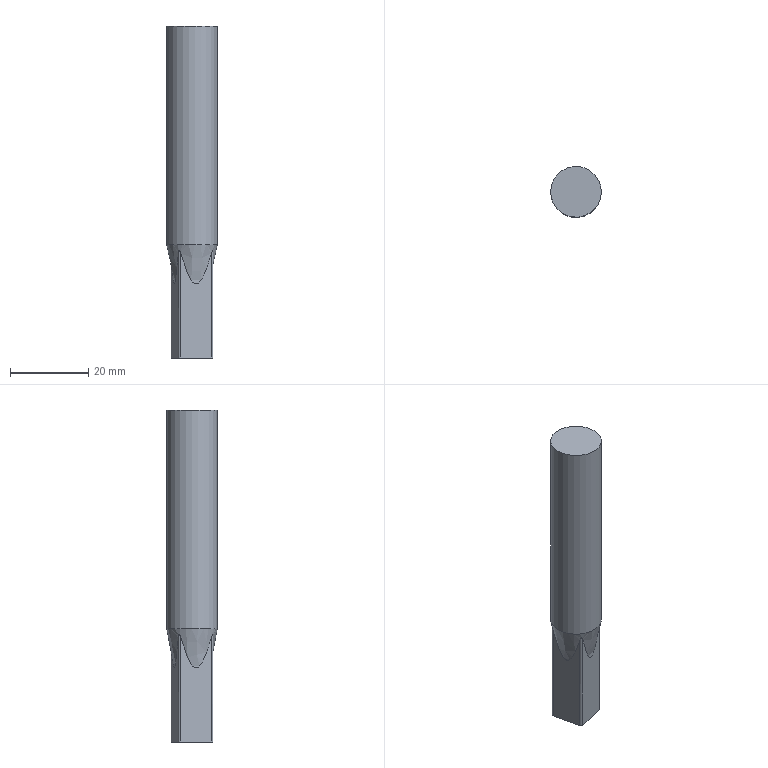Part | NX | features solid 2 | 1 solid | 12 faces | box 13 x 13 x 85 mm | volume 10020 mm3 | plane 6 | cylinder 5 | cone 1 | commonest cylinder face diameters 1.1 x4 13 x1
STEP:
#1=CARTESIAN_POINT('',(-690.242,-351.357,51.));
#2=VERTEX_POINT('',#1);
#3=CARTESIAN_POINT('',(-682.453,-349.534,51.));
#4=VERTEX_POINT('',#3);
#5=CARTESIAN_POINT('',(-686.347,-350.445,51.));
#6=DIRECTION('',(0.9737,0.2278,0.));
#7=VECTOR('',#6,1000.);
#8=LINE('',#5,#7);
#9=EDGE_CURVE('',#2,#4,#8,.T.);
#10=ORIENTED_EDGE('',*,*,#9,.T.);
#11=CARTESIAN_POINT('',(-682.453,-349.534,77.735));
#12=VERTEX_POINT('',#11);
#13=CARTESIAN_POINT('',(-682.453,-349.534,51.));
#14=DIRECTION('',(0.,0.,1.));
#15=VECTOR('',#14,1000.);
#16=LINE('',#13,#15);
#17=EDGE_CURVE('',#4,#12,#16,.T.);
#18=ORIENTED_EDGE('',*,*,#17,.T.);
#19=CARTESIAN_POINT('',(-690.242,-351.357,77.735));
#20=VERTEX_POINT('',#19);
#21=CARTESIAN_POINT('',(-690.242,-351.357,77.735));
#22=CARTESIAN_POINT('',(-690.035,-351.308,77.013));
#23=CARTESIAN_POINT('',(-689.603,-351.207,75.574));
#24=CARTESIAN_POINT('',(-688.992,-351.064,73.795));
#25=CARTESIAN_POINT('',(-688.427,-350.932,72.408));
#26=CARTESIAN_POINT('',(-687.922,-350.814,71.396));
#27=CARTESIAN_POINT('',(-687.342,-350.678,70.456));
#28=CARTESIAN_POINT('',(-686.302,-350.435,69.756));
#29=CARTESIAN_POINT('',(-685.305,-350.201,70.527));
#30=CARTESIAN_POINT('',(-684.739,-350.069,71.456));
#31=CARTESIAN_POINT('',(-684.242,-349.953,72.469));
#32=CARTESIAN_POINT('',(-683.686,-349.823,73.841));
#33=CARTESIAN_POINT('',(-683.085,-349.682,75.597));
#34=CARTESIAN_POINT('',(-682.658,-349.582,77.02));
#35=CARTESIAN_POINT('',(-682.453,-349.534,77.735));
#36=B_SPLINE_CURVE_WITH_KNOTS('',3,(#21,#22,#23,#24,#25,#26,#27,#28,#29,#30,#31,#32,#33,#34,#35),.UNSPECIFIED.,.F.,.F.,(4,1,1,1,1,1,1,1,1,1,1,1,4),(0.002007,0.004266,0.006525,0.007654,0.008784,0.009913,0.01104,0.01217,0.0133,0.01443,0.01556,0.01782,0.02008),.UNSPECIFIED.);
#37=EDGE_CURVE('',#20,#12,#36,.T.);
#38=ORIENTED_EDGE('',*,*,#37,.F.);
#39=CARTESIAN_POINT('',(-690.242,-351.357,51.));
#40=DIRECTION('',(0.,0.,1.));
#41=VECTOR('',#40,1000.);
#42=LINE('',#39,#41);
#43=EDGE_CURVE('',#20,#2,#42,.F.);
#44=ORIENTED_EDGE('',*,*,#43,.T.);
#45=EDGE_LOOP('',(#10,#18,#38,#44));
#46=FACE_BOUND('',#45,.T.);
#47=CARTESIAN_POINT('',(-686.347,-350.445,51.));
#48=DIRECTION('',(0.2278,-0.9737,0.));
#49=DIRECTION('',(0.,0.,-1.));
#50=AXIS2_PLACEMENT_3D('',#47,#48,#49);
#51=PLANE('',#50);
#52=ADVANCED_FACE('',(#46),#51,.T.);
#53=CARTESIAN_POINT('',(-692.726,-343.157,77.735));
#54=VERTEX_POINT('',#53);
#55=CARTESIAN_POINT('',(-690.903,-350.946,77.735));
#56=VERTEX_POINT('',#55);
#57=CARTESIAN_POINT('',(-692.726,-343.157,77.735));
#58=CARTESIAN_POINT('',(-692.677,-343.364,77.013));
#59=CARTESIAN_POINT('',(-692.576,-343.796,75.574));
#60=CARTESIAN_POINT('',(-692.433,-344.407,73.795));
#61=CARTESIAN_POINT('',(-692.301,-344.972,72.408));
#62=CARTESIAN_POINT('',(-692.183,-345.477,71.396));
#63=CARTESIAN_POINT('',(-692.047,-346.057,70.456));
#64=CARTESIAN_POINT('',(-691.804,-347.096,69.756));
#65=CARTESIAN_POINT('',(-691.57,-348.094,70.527));
#66=CARTESIAN_POINT('',(-691.438,-348.66,71.456));
#67=CARTESIAN_POINT('',(-691.322,-349.157,72.469));
#68=CARTESIAN_POINT('',(-691.192,-349.713,73.841));
#69=CARTESIAN_POINT('',(-691.051,-350.314,75.597));
#70=CARTESIAN_POINT('',(-690.951,-350.741,77.02));
#71=CARTESIAN_POINT('',(-690.903,-350.946,77.735));
#72=B_SPLINE_CURVE_WITH_KNOTS('',3,(#57,#58,#59,#60,#61,#62,#63,#64,#65,#66,#67,#68,#69,#70,#71),.UNSPECIFIED.,.F.,.F.,(4,1,1,1,1,1,1,1,1,1,1,1,4),(0.002007,0.004266,0.006525,0.007654,0.008784,0.009913,0.01104,0.01217,0.0133,0.01443,0.01556,0.01782,0.02008),.UNSPECIFIED.);
#73=EDGE_CURVE('',#54,#56,#72,.T.);
#74=ORIENTED_EDGE('',*,*,#73,.F.);
#75=CARTESIAN_POINT('',(-692.726,-343.157,51.));
#76=VERTEX_POINT('',#75);
#77=CARTESIAN_POINT('',(-692.726,-343.157,51.));
#78=DIRECTION('',(0.,0.,1.));
#79=VECTOR('',#78,1000.);
#80=LINE('',#77,#79);
#81=EDGE_CURVE('',#54,#76,#80,.F.);
#82=ORIENTED_EDGE('',*,*,#81,.T.);
#83=CARTESIAN_POINT('',(-690.903,-350.946,51.));
#84=VERTEX_POINT('',#83);
#85=CARTESIAN_POINT('',(-691.814,-347.052,51.));
#86=DIRECTION('',(0.2278,-0.9737,0.));
#87=VECTOR('',#86,1000.);
#88=LINE('',#85,#87);
#89=EDGE_CURVE('',#76,#84,#88,.T.);
#90=ORIENTED_EDGE('',*,*,#89,.T.);
#91=CARTESIAN_POINT('',(-690.903,-350.946,51.));
#92=DIRECTION('',(0.,0.,1.));
#93=VECTOR('',#92,1000.);
#94=LINE('',#91,#93);
#95=EDGE_CURVE('',#84,#56,#94,.T.);
#96=ORIENTED_EDGE('',*,*,#95,.T.);
#97=EDGE_LOOP('',(#74,#82,#90,#96));
#98=FACE_BOUND('',#97,.T.);
#99=CARTESIAN_POINT('',(-691.814,-347.052,51.));
#100=DIRECTION('',(-0.9737,-0.2278,0.));
#101=DIRECTION('',(0.,0.,1.));
#102=AXIS2_PLACEMENT_3D('',#99,#100,#101);
#103=PLANE('',#102);
#104=ADVANCED_FACE('',(#98),#103,.T.);
#105=CARTESIAN_POINT('',(-684.526,-340.673,77.735));
#106=VERTEX_POINT('',#105);
#107=CARTESIAN_POINT('',(-692.315,-342.496,77.735));
#108=VERTEX_POINT('',#107);
#109=CARTESIAN_POINT('',(-684.526,-340.673,77.735));
#110=CARTESIAN_POINT('',(-684.733,-340.722,77.013));
#111=CARTESIAN_POINT('',(-685.165,-340.823,75.574));
#112=CARTESIAN_POINT('',(-685.776,-340.966,73.795));
#113=CARTESIAN_POINT('',(-686.341,-341.098,72.408));
#114=CARTESIAN_POINT('',(-686.846,-341.216,71.396));
#115=CARTESIAN_POINT('',(-687.426,-341.352,70.456));
#116=CARTESIAN_POINT('',(-688.465,-341.595,69.756));
#117=CARTESIAN_POINT('',(-689.463,-341.829,70.527));
#118=CARTESIAN_POINT('',(-690.029,-341.961,71.456));
#119=CARTESIAN_POINT('',(-690.526,-342.077,72.469));
#120=CARTESIAN_POINT('',(-691.082,-342.207,73.841));
#121=CARTESIAN_POINT('',(-691.683,-342.348,75.597));
#122=CARTESIAN_POINT('',(-692.11,-342.448,77.02));
#123=CARTESIAN_POINT('',(-692.315,-342.496,77.735));
#124=B_SPLINE_CURVE_WITH_KNOTS('',3,(#109,#110,#111,#112,#113,#114,#115,#116,#117,#118,#119,#120,#121,#122,#123),.UNSPECIFIED.,.F.,.F.,(4,1,1,1,1,1,1,1,1,1,1,1,4),(0.002007,0.004266,0.006525,0.007654,0.008784,0.009913,0.01104,0.01217,0.0133,0.01443,0.01556,0.01782,0.02008),.UNSPECIFIED.);
#125=EDGE_CURVE('',#106,#108,#124,.T.);
#126=ORIENTED_EDGE('',*,*,#125,.F.);
#127=CARTESIAN_POINT('',(-684.526,-340.673,51.));
#128=VERTEX_POINT('',#127);
#129=CARTESIAN_POINT('',(-684.526,-340.673,51.));
#130=DIRECTION('',(0.,0.,1.));
#131=VECTOR('',#130,1000.);
#132=LINE('',#129,#131);
#133=EDGE_CURVE('',#106,#128,#132,.F.);
#134=ORIENTED_EDGE('',*,*,#133,.T.);
#135=CARTESIAN_POINT('',(-692.315,-342.496,51.));
#136=VERTEX_POINT('',#135);
#137=CARTESIAN_POINT('',(-688.421,-341.585,51.));
#138=DIRECTION('',(-0.9737,-0.2278,0.));
#139=VECTOR('',#138,1000.);
#140=LINE('',#137,#139);
#141=EDGE_CURVE('',#128,#136,#140,.T.);
#142=ORIENTED_EDGE('',*,*,#141,.T.);
#143=CARTESIAN_POINT('',(-692.315,-342.496,51.));
#144=DIRECTION('',(0.,0.,1.));
#145=VECTOR('',#144,1000.);
#146=LINE('',#143,#145);
#147=EDGE_CURVE('',#136,#108,#146,.T.);
#148=ORIENTED_EDGE('',*,*,#147,.T.);
#149=EDGE_LOOP('',(#126,#134,#142,#148));
#150=FACE_BOUND('',#149,.T.);
#151=CARTESIAN_POINT('',(-688.421,-341.585,51.));
#152=DIRECTION('',(-0.2278,0.9737,0.));
#153=DIRECTION('',(0.,0.,1.));
#154=AXIS2_PLACEMENT_3D('',#151,#152,#153);
#155=PLANE('',#154);
#156=ADVANCED_FACE('',(#150),#155,.T.);
#157=CARTESIAN_POINT('',(-682.042,-348.873,51.));
#158=VERTEX_POINT('',#157);
#159=CARTESIAN_POINT('',(-683.865,-341.084,51.));
#160=VERTEX_POINT('',#159);
#161=CARTESIAN_POINT('',(-682.954,-344.978,51.));
#162=DIRECTION('',(-0.2278,0.9737,0.));
#163=VECTOR('',#162,1000.);
#164=LINE('',#161,#163);
#165=EDGE_CURVE('',#158,#160,#164,.T.);
#166=ORIENTED_EDGE('',*,*,#165,.F.);
#167=CARTESIAN_POINT('',(-682.578,-348.998,51.));
#168=DIRECTION('',(0.,0.,-1.));
#169=DIRECTION('',(-1.,0.,0.));
#170=AXIS2_PLACEMENT_3D('',#167,#168,#169);
#171=CIRCLE('',#170,0.55);
#172=EDGE_CURVE('',#158,#4,#171,.T.);
#173=ORIENTED_EDGE('',*,*,#172,.T.);
#174=ORIENTED_EDGE('',*,*,#9,.F.);
#175=CARTESIAN_POINT('',(-690.367,-350.821,51.));
#176=DIRECTION('',(0.,0.,-1.));
#177=DIRECTION('',(-1.,0.,0.));
#178=AXIS2_PLACEMENT_3D('',#175,#176,#177);
#179=CIRCLE('',#178,0.55);
#180=EDGE_CURVE('',#2,#84,#179,.T.);
#181=ORIENTED_EDGE('',*,*,#180,.T.);
#182=ORIENTED_EDGE('',*,*,#89,.F.);
#183=CARTESIAN_POINT('',(-692.19,-343.031,51.));
#184=DIRECTION('',(0.,0.,-1.));
#185=DIRECTION('',(-1.,0.,0.));
#186=AXIS2_PLACEMENT_3D('',#183,#184,#185);
#187=CIRCLE('',#186,0.55);
#188=EDGE_CURVE('',#76,#136,#187,.T.);
#189=ORIENTED_EDGE('',*,*,#188,.T.);
#190=ORIENTED_EDGE('',*,*,#141,.F.);
#191=CARTESIAN_POINT('',(-684.4,-341.209,51.));
#192=DIRECTION('',(0.,0.,-1.));
#193=DIRECTION('',(-1.,0.,0.));
#194=AXIS2_PLACEMENT_3D('',#191,#192,#193);
#195=CIRCLE('',#194,0.55);
#196=EDGE_CURVE('',#128,#160,#195,.T.);
#197=ORIENTED_EDGE('',*,*,#196,.T.);
#198=EDGE_LOOP('',(#166,#173,#174,#181,#182,#189,#190,#197));
#199=FACE_BOUND('',#198,.T.);
#200=CARTESIAN_POINT('',(-687.384,-346.015,51.));
#201=DIRECTION('',(0.,0.,-1.));
#202=DIRECTION('',(-0.9737,-0.2278,0.));
#203=AXIS2_PLACEMENT_3D('',#200,#201,#202);
#204=PLANE('',#203);
#205=ADVANCED_FACE('',(#199),#204,.T.);
#206=CARTESIAN_POINT('',(-682.042,-348.873,77.735));
#207=VERTEX_POINT('',#206);
#208=CARTESIAN_POINT('',(-683.865,-341.084,77.735));
#209=VERTEX_POINT('',#208);
#210=CARTESIAN_POINT('',(-682.042,-348.873,77.735));
#211=CARTESIAN_POINT('',(-682.091,-348.666,77.013));
#212=CARTESIAN_POINT('',(-682.192,-348.234,75.574));
#213=CARTESIAN_POINT('',(-682.335,-347.623,73.795));
#214=CARTESIAN_POINT('',(-682.467,-347.058,72.408));
#215=CARTESIAN_POINT('',(-682.585,-346.553,71.396));
#216=CARTESIAN_POINT('',(-682.721,-345.973,70.456));
#217=CARTESIAN_POINT('',(-682.964,-344.933,69.756));
#218=CARTESIAN_POINT('',(-683.198,-343.936,70.527));
#219=CARTESIAN_POINT('',(-683.33,-343.37,71.456));
#220=CARTESIAN_POINT('',(-683.446,-342.873,72.469));
#221=CARTESIAN_POINT('',(-683.576,-342.317,73.841));
#222=CARTESIAN_POINT('',(-683.717,-341.716,75.597));
#223=CARTESIAN_POINT('',(-683.817,-341.289,77.02));
#224=CARTESIAN_POINT('',(-683.865,-341.084,77.735));
#225=B_SPLINE_CURVE_WITH_KNOTS('',3,(#210,#211,#212,#213,#214,#215,#216,#217,#218,#219,#220,#221,#222,#223,#224),.UNSPECIFIED.,.F.,.F.,(4,1,1,1,1,1,1,1,1,1,1,1,4),(0.002007,0.004266,0.006525,0.007654,0.008784,0.009913,0.01104,0.01217,0.0133,0.01443,0.01556,0.01782,0.02008),.UNSPECIFIED.);
#226=EDGE_CURVE('',#207,#209,#225,.T.);
#227=ORIENTED_EDGE('',*,*,#226,.F.);
#228=CARTESIAN_POINT('',(-682.042,-348.873,51.));
#229=DIRECTION('',(0.,0.,1.));
#230=VECTOR('',#229,1000.);
#231=LINE('',#228,#230);
#232=EDGE_CURVE('',#207,#158,#231,.F.);
#233=ORIENTED_EDGE('',*,*,#232,.T.);
#234=ORIENTED_EDGE('',*,*,#165,.T.);
#235=CARTESIAN_POINT('',(-683.865,-341.084,51.));
#236=DIRECTION('',(0.,0.,1.));
#237=VECTOR('',#236,1000.);
#238=LINE('',#235,#237);
#239=EDGE_CURVE('',#160,#209,#238,.T.);
#240=ORIENTED_EDGE('',*,*,#239,.T.);
#241=EDGE_LOOP('',(#227,#233,#234,#240));
#242=FACE_BOUND('',#241,.T.);
#243=CARTESIAN_POINT('',(-682.954,-344.978,51.));
#244=DIRECTION('',(0.9737,0.2278,0.));
#245=DIRECTION('',(0.,0.,-1.));
#246=AXIS2_PLACEMENT_3D('',#243,#244,#245);
#247=PLANE('',#246);
#248=ADVANCED_FACE('',(#242),#247,.T.);
#249=ORIENTED_EDGE('',*,*,#226,.T.);
#250=CARTESIAN_POINT('',(-683.865,-341.084,77.735));
#251=CARTESIAN_POINT('',(-683.875,-341.042,77.881));
#252=CARTESIAN_POINT('',(-683.901,-340.971,78.1));
#253=CARTESIAN_POINT('',(-683.962,-340.866,78.368));
#254=CARTESIAN_POINT('',(-684.105,-340.728,78.562));
#255=CARTESIAN_POINT('',(-684.29,-340.664,78.363));
#256=CARTESIAN_POINT('',(-684.409,-340.656,78.099));
#257=CARTESIAN_POINT('',(-684.484,-340.664,77.88));
#258=CARTESIAN_POINT('',(-684.526,-340.673,77.735));
#259=B_SPLINE_CURVE_WITH_KNOTS('',3,(#250,#251,#252,#253,#254,#255,#256,#257,#258),.UNSPECIFIED.,.F.,.F.,(4,1,1,1,1,1,4),(0.,0.0004558,0.0006837,0.0009116,0.001139,0.001367,0.001823),.UNSPECIFIED.);
#260=EDGE_CURVE('',#209,#106,#259,.T.);
#261=ORIENTED_EDGE('',*,*,#260,.T.);
#262=ORIENTED_EDGE('',*,*,#125,.T.);
#263=CARTESIAN_POINT('',(-692.315,-342.496,77.735));
#264=CARTESIAN_POINT('',(-692.357,-342.506,77.881));
#265=CARTESIAN_POINT('',(-692.428,-342.532,78.1));
#266=CARTESIAN_POINT('',(-692.533,-342.593,78.368));
#267=CARTESIAN_POINT('',(-692.671,-342.736,78.562));
#268=CARTESIAN_POINT('',(-692.735,-342.921,78.363));
#269=CARTESIAN_POINT('',(-692.743,-343.04,78.099));
#270=CARTESIAN_POINT('',(-692.735,-343.115,77.88));
#271=CARTESIAN_POINT('',(-692.726,-343.157,77.735));
#272=B_SPLINE_CURVE_WITH_KNOTS('',3,(#263,#264,#265,#266,#267,#268,#269,#270,#271),.UNSPECIFIED.,.F.,.F.,(4,1,1,1,1,1,4),(0.,0.0004558,0.0006837,0.0009116,0.001139,0.001367,0.001823),.UNSPECIFIED.);
#273=EDGE_CURVE('',#108,#54,#272,.T.);
#274=ORIENTED_EDGE('',*,*,#273,.T.);
#275=ORIENTED_EDGE('',*,*,#73,.T.);
#276=CARTESIAN_POINT('',(-690.903,-350.946,77.735));
#277=CARTESIAN_POINT('',(-690.893,-350.988,77.881));
#278=CARTESIAN_POINT('',(-690.867,-351.059,78.1));
#279=CARTESIAN_POINT('',(-690.806,-351.164,78.368));
#280=CARTESIAN_POINT('',(-690.663,-351.302,78.562));
#281=CARTESIAN_POINT('',(-690.478,-351.366,78.363));
#282=CARTESIAN_POINT('',(-690.359,-351.374,78.099));
#283=CARTESIAN_POINT('',(-690.284,-351.366,77.88));
#284=CARTESIAN_POINT('',(-690.242,-351.357,77.735));
#285=B_SPLINE_CURVE_WITH_KNOTS('',3,(#276,#277,#278,#279,#280,#281,#282,#283,#284),.UNSPECIFIED.,.F.,.F.,(4,1,1,1,1,1,4),(0.,0.0004558,0.0006837,0.0009116,0.001139,0.001367,0.001823),.UNSPECIFIED.);
#286=EDGE_CURVE('',#56,#20,#285,.T.);
#287=ORIENTED_EDGE('',*,*,#286,.T.);
#288=ORIENTED_EDGE('',*,*,#37,.T.);
#289=CARTESIAN_POINT('',(-682.453,-349.534,77.735));
#290=CARTESIAN_POINT('',(-682.411,-349.524,77.881));
#291=CARTESIAN_POINT('',(-682.34,-349.498,78.1));
#292=CARTESIAN_POINT('',(-682.235,-349.437,78.368));
#293=CARTESIAN_POINT('',(-682.097,-349.294,78.562));
#294=CARTESIAN_POINT('',(-682.033,-349.109,78.363));
#295=CARTESIAN_POINT('',(-682.025,-348.99,78.099));
#296=CARTESIAN_POINT('',(-682.033,-348.915,77.88));
#297=CARTESIAN_POINT('',(-682.042,-348.873,77.735));
#298=B_SPLINE_CURVE_WITH_KNOTS('',3,(#289,#290,#291,#292,#293,#294,#295,#296,#297),.UNSPECIFIED.,.F.,.F.,(4,1,1,1,1,1,4),(0.,0.0004558,0.0006837,0.0009116,0.001139,0.001367,0.001823),.UNSPECIFIED.);
#299=EDGE_CURVE('',#12,#207,#298,.T.);
#300=ORIENTED_EDGE('',*,*,#299,.T.);
#301=EDGE_LOOP('',(#249,#261,#262,#274,#275,#287,#288,#300));
#302=FACE_BOUND('',#301,.T.);
#303=CARTESIAN_POINT('',(-681.055,-344.534,80.));
#304=VERTEX_POINT('',#303);
#305=CARTESIAN_POINT('',(-687.384,-346.015,80.));
#306=DIRECTION('',(0.,0.,1.));
#307=DIRECTION('',(0.9737,0.2278,0.));
#308=AXIS2_PLACEMENT_3D('',#305,#306,#307);
#309=CIRCLE('',#308,6.5);
#310=EDGE_CURVE('',#304,#304,#309,.T.);
#311=ORIENTED_EDGE('',*,*,#310,.F.);
#312=EDGE_LOOP('',(#311));
#313=FACE_BOUND('',#312,.T.);
#314=CARTESIAN_POINT('',(-687.384,-346.015,70.));
#315=DIRECTION('',(0.,0.,1.));
#316=DIRECTION('',(0.9737,0.2278,0.));
#317=AXIS2_PLACEMENT_3D('',#314,#315,#316);
#318=CONICAL_SURFACE('',#317,4.55,0.1926);
#319=ADVANCED_FACE('',(#302,#313),#318,.T.);
#320=CARTESIAN_POINT('',(-693.713,-347.496,136.));
#321=VERTEX_POINT('',#320);
#322=CARTESIAN_POINT('',(-687.384,-346.015,136.));
#323=DIRECTION('',(0.,0.,-1.));
#324=DIRECTION('',(-0.9737,-0.2278,0.));
#325=AXIS2_PLACEMENT_3D('',#322,#323,#324);
#326=CIRCLE('',#325,6.5);
#327=EDGE_CURVE('',#321,#321,#326,.T.);
#328=ORIENTED_EDGE('',*,*,#327,.F.);
#329=EDGE_LOOP('',(#328));
#330=FACE_BOUND('',#329,.T.);
#331=CARTESIAN_POINT('',(-687.384,-346.015,136.));
#332=DIRECTION('',(0.,0.,1.));
#333=DIRECTION('',(0.9737,0.2278,0.));
#334=AXIS2_PLACEMENT_3D('',#331,#332,#333);
#335=PLANE('',#334);
#336=ADVANCED_FACE('',(#330),#335,.T.);
#337=ORIENTED_EDGE('',*,*,#327,.T.);
#338=EDGE_LOOP('',(#337));
#339=FACE_BOUND('',#338,.T.);
#340=ORIENTED_EDGE('',*,*,#310,.T.);
#341=EDGE_LOOP('',(#340));
#342=FACE_BOUND('',#341,.T.);
#343=CARTESIAN_POINT('',(-687.384,-346.015,80.));
#344=DIRECTION('',(0.,0.,1.));
#345=DIRECTION('',(0.9737,0.2278,0.));
#346=AXIS2_PLACEMENT_3D('',#343,#344,#345);
#347=CYLINDRICAL_SURFACE('',#346,6.5);
#348=ADVANCED_FACE('',(#339,#342),#347,.T.);
#349=ORIENTED_EDGE('',*,*,#172,.F.);
#350=ORIENTED_EDGE('',*,*,#232,.F.);
#351=ORIENTED_EDGE('',*,*,#299,.F.);
#352=ORIENTED_EDGE('',*,*,#17,.F.);
#353=EDGE_LOOP('',(#349,#350,#351,#352));
#354=FACE_BOUND('',#353,.T.);
#355=CARTESIAN_POINT('',(-682.578,-348.998,51.));
#356=DIRECTION('',(0.,0.,1.));
#357=DIRECTION('',(1.,0.,0.));
#358=AXIS2_PLACEMENT_3D('',#355,#356,#357);
#359=CYLINDRICAL_SURFACE('',#358,0.55);
#360=ADVANCED_FACE('',(#354),#359,.T.);
#361=ORIENTED_EDGE('',*,*,#196,.F.);
#362=ORIENTED_EDGE('',*,*,#133,.F.);
#363=ORIENTED_EDGE('',*,*,#260,.F.);
#364=ORIENTED_EDGE('',*,*,#239,.F.);
#365=EDGE_LOOP('',(#361,#362,#363,#364));
#366=FACE_BOUND('',#365,.T.);
#367=CARTESIAN_POINT('',(-684.4,-341.209,51.));
#368=DIRECTION('',(0.,0.,1.));
#369=DIRECTION('',(1.,0.,0.));
#370=AXIS2_PLACEMENT_3D('',#367,#368,#369);
#371=CYLINDRICAL_SURFACE('',#370,0.55);
#372=ADVANCED_FACE('',(#366),#371,.T.);
#373=ORIENTED_EDGE('',*,*,#188,.F.);
#374=ORIENTED_EDGE('',*,*,#81,.F.);
#375=ORIENTED_EDGE('',*,*,#273,.F.);
#376=ORIENTED_EDGE('',*,*,#147,.F.);
#377=EDGE_LOOP('',(#373,#374,#375,#376));
#378=FACE_BOUND('',#377,.T.);
#379=CARTESIAN_POINT('',(-692.19,-343.031,51.));
#380=DIRECTION('',(0.,0.,1.));
#381=DIRECTION('',(1.,0.,0.));
#382=AXIS2_PLACEMENT_3D('',#379,#380,#381);
#383=CYLINDRICAL_SURFACE('',#382,0.55);
#384=ADVANCED_FACE('',(#378),#383,.T.);
#385=ORIENTED_EDGE('',*,*,#180,.F.);
#386=ORIENTED_EDGE('',*,*,#43,.F.);
#387=ORIENTED_EDGE('',*,*,#286,.F.);
#388=ORIENTED_EDGE('',*,*,#95,.F.);
#389=EDGE_LOOP('',(#385,#386,#387,#388));
#390=FACE_BOUND('',#389,.T.);
#391=CARTESIAN_POINT('',(-690.367,-350.821,51.));
#392=DIRECTION('',(0.,0.,1.));
#393=DIRECTION('',(1.,0.,0.));
#394=AXIS2_PLACEMENT_3D('',#391,#392,#393);
#395=CYLINDRICAL_SURFACE('',#394,0.55);
#396=ADVANCED_FACE('',(#390),#395,.T.);
#397=CLOSED_SHELL('',(#52,#104,#156,#205,#248,#319,#336,#348,#360,#372,#384,#396));
#398=MANIFOLD_SOLID_BREP('',#397);
#399=(LENGTH_UNIT()NAMED_UNIT(*)SI_UNIT(.MILLI.,.METRE.));
#400=UNCERTAINTY_MEASURE_WITH_UNIT(LENGTH_MEASURE(0.0508),#399,'','');
#401=(NAMED_UNIT(*)PLANE_ANGLE_UNIT()SI_UNIT($,.RADIAN.));
#402=(NAMED_UNIT(*)SI_UNIT($,.STERADIAN.)SOLID_ANGLE_UNIT());
#403=(GEOMETRIC_REPRESENTATION_CONTEXT(3)GLOBAL_UNCERTAINTY_ASSIGNED_CONTEXT((#400))GLOBAL_UNIT_ASSIGNED_CONTEXT((#399,#401,#402))REPRESENTATION_CONTEXT('',''));
#404=ADVANCED_BREP_SHAPE_REPRESENTATION('',(#398),#403);